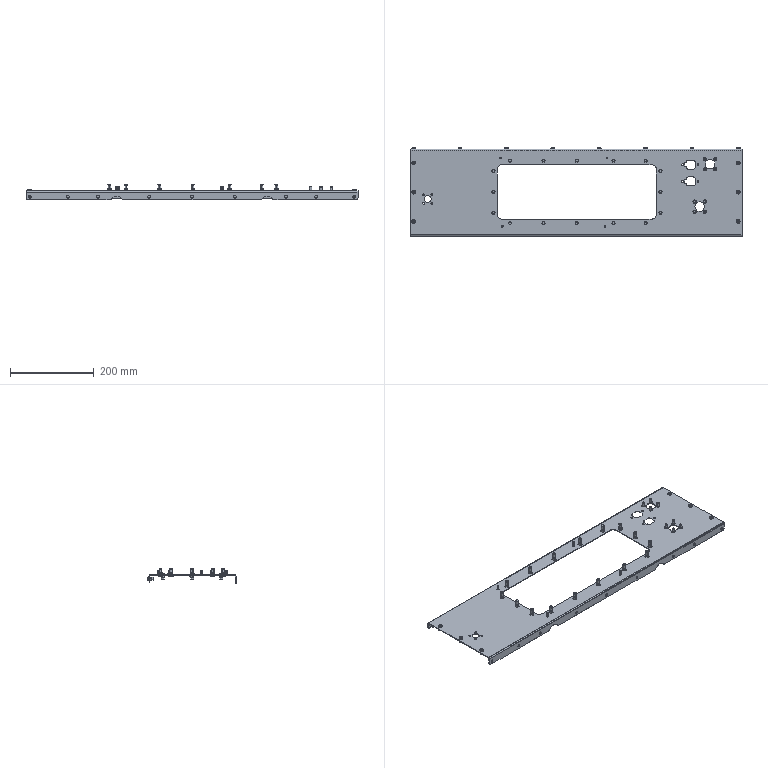Part | NX | features BREP 5 | 43 solids | 1548 faces | box 795 x 210.8 x 37.5 mm | volume 220520 mm3 | plane 760 | cylinder 508 | cone 232 | spline 48 | commonest cylinder face diameters 4 x120 6.2 x60 10 x36 5 x32 6.9 x32 4.2 x28